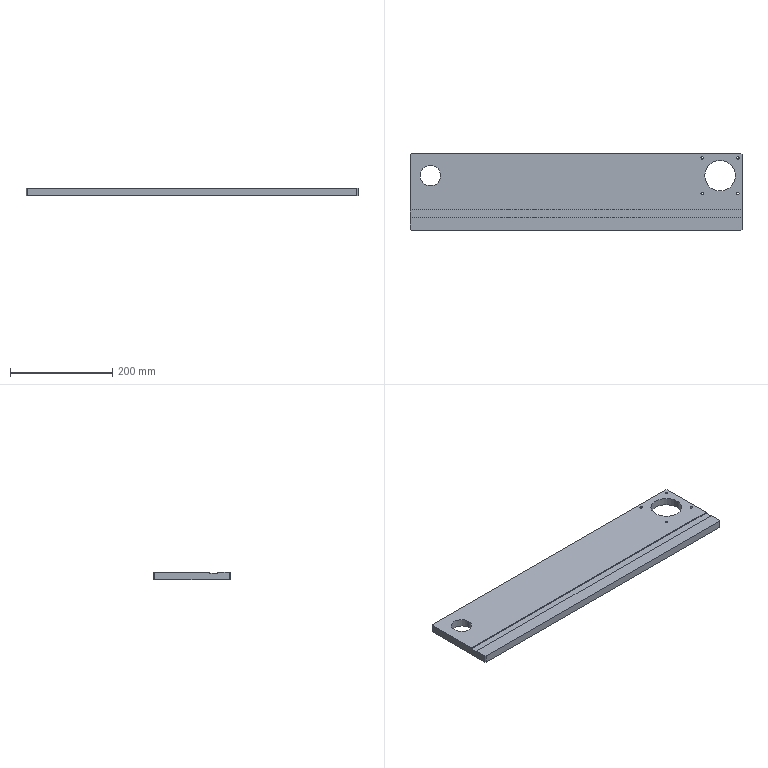Part | STEP file | 001-010-Mounting vertical plate | 1 solid | 26 faces | box 650 x 150 x 15 mm | volume 1380441 mm3 | plane 14 | cylinder 12 | commonest cylinder face diameters 5 x8 40 x2 60 x2